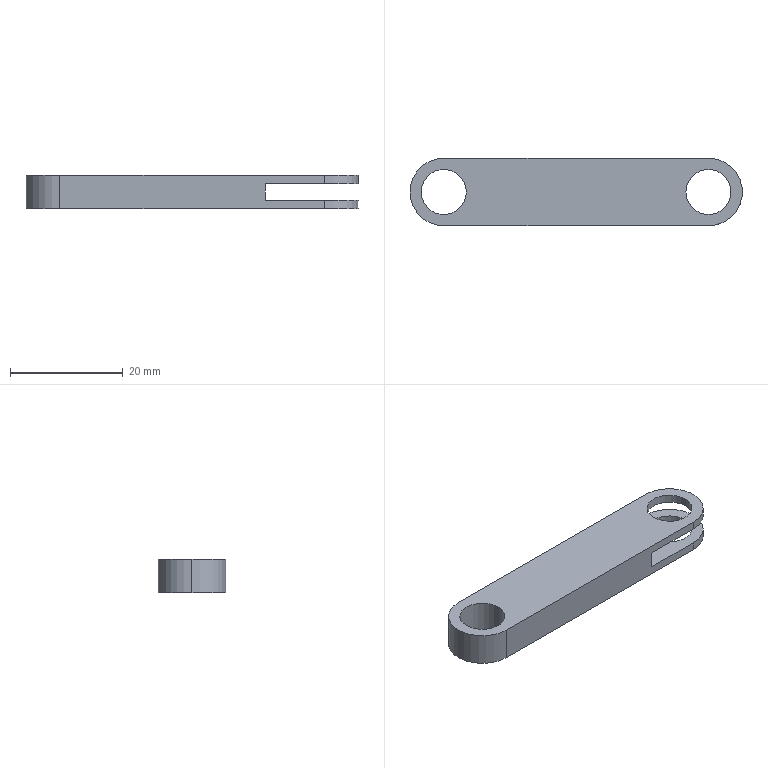Part | SolidWorks | features ICE 2, Extrusion 1 | 1 solid | 17 faces | box 59 x 12 x 6 mm | volume 3063 mm3 | cylinder 10 | plane 7 | commonest cylinder face diameters 8 x6 12 x4
STEP:
#1=CARTESIAN_POINT('',(-27.5,0.,0.));
#2=VERTEX_POINT('',#1);
#3=CARTESIAN_POINT('',(-19.5,0.,0.));
#4=VERTEX_POINT('',#3);
#5=CARTESIAN_POINT('',(-23.5,0.,0.));
#6=DIRECTION('',(0.,0.,1.));
#7=DIRECTION('',(1.,0.,0.));
#8=AXIS2_PLACEMENT_3D('',#5,#6,#7);
#9=CIRCLE('',#8,4.);
#10=EDGE_CURVE('',#2,#4,#9,.T.);
#11=ORIENTED_EDGE('',*,*,#10,.F.);
#12=CARTESIAN_POINT('',(-27.5,0.,6.));
#13=VERTEX_POINT('',#12);
#14=CARTESIAN_POINT('',(-27.5,0.,-29.));
#15=DIRECTION('',(0.,0.,1.));
#16=VECTOR('',#15,1000.);
#17=LINE('',#14,#16);
#18=EDGE_CURVE('',#2,#13,#17,.T.);
#19=ORIENTED_EDGE('',*,*,#18,.T.);
#20=CARTESIAN_POINT('',(-19.5,0.,6.));
#21=VERTEX_POINT('',#20);
#22=CARTESIAN_POINT('',(-23.5,0.,6.));
#23=DIRECTION('',(0.,0.,1.));
#24=DIRECTION('',(1.,0.,0.));
#25=AXIS2_PLACEMENT_3D('',#22,#23,#24);
#26=CIRCLE('',#25,4.);
#27=EDGE_CURVE('',#13,#21,#26,.T.);
#28=ORIENTED_EDGE('',*,*,#27,.T.);
#29=CARTESIAN_POINT('',(-19.5,0.,-29.));
#30=DIRECTION('',(0.,0.,1.));
#31=VECTOR('',#30,1000.);
#32=LINE('',#29,#31);
#33=EDGE_CURVE('',#4,#21,#32,.T.);
#34=ORIENTED_EDGE('',*,*,#33,.F.);
#35=EDGE_LOOP('',(#11,#19,#28,#34));
#36=FACE_OUTER_BOUND('',#35,.T.);
#37=CARTESIAN_POINT('',(-23.5,0.,-29.));
#38=DIRECTION('',(0.,0.,1.));
#39=DIRECTION('',(1.,0.,0.));
#40=AXIS2_PLACEMENT_3D('',#37,#38,#39);
#41=CYLINDRICAL_SURFACE('',#40,4.);
#42=ADVANCED_FACE('',(#36),#41,.F.);
#43=CARTESIAN_POINT('',(19.5,0.,4.5));
#44=VERTEX_POINT('',#43);
#45=CARTESIAN_POINT('',(27.5,0.,4.5));
#46=VERTEX_POINT('',#45);
#47=CARTESIAN_POINT('',(23.5,0.,4.5));
#48=DIRECTION('',(0.,0.,1.));
#49=DIRECTION('',(1.,0.,0.));
#50=AXIS2_PLACEMENT_3D('',#47,#48,#49);
#51=CIRCLE('',#50,4.);
#52=EDGE_CURVE('',#44,#46,#51,.T.);
#53=ORIENTED_EDGE('',*,*,#52,.F.);
#54=CARTESIAN_POINT('',(19.5,0.,6.));
#55=VERTEX_POINT('',#54);
#56=CARTESIAN_POINT('',(19.5,0.,-29.));
#57=DIRECTION('',(0.,0.,1.));
#58=VECTOR('',#57,1000.);
#59=LINE('',#56,#58);
#60=EDGE_CURVE('',#44,#55,#59,.T.);
#61=ORIENTED_EDGE('',*,*,#60,.T.);
#62=CARTESIAN_POINT('',(27.5,0.,6.));
#63=VERTEX_POINT('',#62);
#64=CARTESIAN_POINT('',(23.5,0.,6.));
#65=DIRECTION('',(0.,0.,1.));
#66=DIRECTION('',(1.,0.,0.));
#67=AXIS2_PLACEMENT_3D('',#64,#65,#66);
#68=CIRCLE('',#67,4.);
#69=EDGE_CURVE('',#55,#63,#68,.T.);
#70=ORIENTED_EDGE('',*,*,#69,.T.);
#71=CARTESIAN_POINT('',(27.5,0.,-29.));
#72=DIRECTION('',(0.,0.,1.));
#73=VECTOR('',#72,1000.);
#74=LINE('',#71,#73);
#75=EDGE_CURVE('',#46,#63,#74,.T.);
#76=ORIENTED_EDGE('',*,*,#75,.F.);
#77=EDGE_LOOP('',(#53,#61,#70,#76));
#78=FACE_OUTER_BOUND('',#77,.T.);
#79=CARTESIAN_POINT('',(23.5,0.,-29.));
#80=DIRECTION('',(0.,0.,1.));
#81=DIRECTION('',(1.,0.,0.));
#82=AXIS2_PLACEMENT_3D('',#79,#80,#81);
#83=CYLINDRICAL_SURFACE('',#82,4.);
#84=ADVANCED_FACE('',(#78),#83,.F.);
#85=CARTESIAN_POINT('',(19.5,0.,0.));
#86=VERTEX_POINT('',#85);
#87=CARTESIAN_POINT('',(27.5,0.,0.));
#88=VERTEX_POINT('',#87);
#89=CARTESIAN_POINT('',(23.5,0.,0.));
#90=DIRECTION('',(0.,0.,1.));
#91=DIRECTION('',(1.,0.,0.));
#92=AXIS2_PLACEMENT_3D('',#89,#90,#91);
#93=CIRCLE('',#92,4.);
#94=EDGE_CURVE('',#86,#88,#93,.T.);
#95=ORIENTED_EDGE('',*,*,#94,.F.);
#96=CARTESIAN_POINT('',(19.5,0.,1.5));
#97=VERTEX_POINT('',#96);
#98=CARTESIAN_POINT('',(19.5,0.,-29.));
#99=DIRECTION('',(0.,0.,1.));
#100=VECTOR('',#99,1000.);
#101=LINE('',#98,#100);
#102=EDGE_CURVE('',#86,#97,#101,.T.);
#103=ORIENTED_EDGE('',*,*,#102,.T.);
#104=CARTESIAN_POINT('',(27.5,0.,1.5));
#105=VERTEX_POINT('',#104);
#106=CARTESIAN_POINT('',(23.5,0.,1.5));
#107=DIRECTION('',(0.,0.,-1.));
#108=DIRECTION('',(-1.,0.,0.));
#109=AXIS2_PLACEMENT_3D('',#106,#107,#108);
#110=CIRCLE('',#109,4.);
#111=EDGE_CURVE('',#105,#97,#110,.T.);
#112=ORIENTED_EDGE('',*,*,#111,.F.);
#113=CARTESIAN_POINT('',(27.5,0.,-29.));
#114=DIRECTION('',(0.,0.,1.));
#115=VECTOR('',#114,1000.);
#116=LINE('',#113,#115);
#117=EDGE_CURVE('',#88,#105,#116,.T.);
#118=ORIENTED_EDGE('',*,*,#117,.F.);
#119=EDGE_LOOP('',(#95,#103,#112,#118));
#120=FACE_OUTER_BOUND('',#119,.T.);
#121=CARTESIAN_POINT('',(23.5,0.,-29.));
#122=DIRECTION('',(0.,0.,1.));
#123=DIRECTION('',(1.,0.,0.));
#124=AXIS2_PLACEMENT_3D('',#121,#122,#123);
#125=CYLINDRICAL_SURFACE('',#124,4.);
#126=ADVANCED_FACE('',(#120),#125,.F.);
#127=CARTESIAN_POINT('',(-29.5,0.,6.));
#128=VERTEX_POINT('',#127);
#129=CARTESIAN_POINT('',(-23.5,-6.,6.));
#130=VERTEX_POINT('',#129);
#131=CARTESIAN_POINT('',(-23.5,0.,6.));
#132=DIRECTION('',(0.,0.,1.));
#133=DIRECTION('',(1.,0.,0.));
#134=AXIS2_PLACEMENT_3D('',#131,#132,#133);
#135=CIRCLE('',#134,6.);
#136=EDGE_CURVE('',#128,#130,#135,.T.);
#137=ORIENTED_EDGE('',*,*,#136,.F.);
#138=CARTESIAN_POINT('',(-29.5,0.,0.));
#139=VERTEX_POINT('',#138);
#140=CARTESIAN_POINT('',(-29.5,0.,6.));
#141=DIRECTION('',(0.,0.,-1.));
#142=VECTOR('',#141,1000.);
#143=LINE('',#140,#142);
#144=EDGE_CURVE('',#128,#139,#143,.T.);
#145=ORIENTED_EDGE('',*,*,#144,.T.);
#146=CARTESIAN_POINT('',(-23.5,-6.,0.));
#147=VERTEX_POINT('',#146);
#148=CARTESIAN_POINT('',(-23.5,0.,0.));
#149=DIRECTION('',(0.,0.,1.));
#150=DIRECTION('',(1.,0.,0.));
#151=AXIS2_PLACEMENT_3D('',#148,#149,#150);
#152=CIRCLE('',#151,6.);
#153=EDGE_CURVE('',#139,#147,#152,.T.);
#154=ORIENTED_EDGE('',*,*,#153,.T.);
#155=CARTESIAN_POINT('',(-23.5,-6.,6.));
#156=DIRECTION('',(0.,0.,-1.));
#157=VECTOR('',#156,1000.);
#158=LINE('',#155,#157);
#159=EDGE_CURVE('',#130,#147,#158,.T.);
#160=ORIENTED_EDGE('',*,*,#159,.F.);
#161=EDGE_LOOP('',(#137,#145,#154,#160));
#162=FACE_OUTER_BOUND('',#161,.T.);
#163=CARTESIAN_POINT('',(-23.5,0.,6.));
#164=DIRECTION('',(0.,0.,-1.));
#165=DIRECTION('',(-1.,0.,0.));
#166=AXIS2_PLACEMENT_3D('',#163,#164,#165);
#167=CYLINDRICAL_SURFACE('',#166,6.);
#168=ADVANCED_FACE('',(#162),#167,.T.);
#169=CARTESIAN_POINT('',(23.5,-6.,6.));
#170=VERTEX_POINT('',#169);
#171=CARTESIAN_POINT('',(23.5,-6.,4.5));
#172=VERTEX_POINT('',#171);
#173=CARTESIAN_POINT('',(23.5,-6.,6.));
#174=DIRECTION('',(0.,0.,-1.));
#175=VECTOR('',#174,1000.);
#176=LINE('',#173,#175);
#177=EDGE_CURVE('',#170,#172,#176,.T.);
#178=ORIENTED_EDGE('',*,*,#177,.T.);
#179=CARTESIAN_POINT('',(23.5,6.,4.5));
#180=VERTEX_POINT('',#179);
#181=CARTESIAN_POINT('',(23.5,0.,4.5));
#182=DIRECTION('',(0.,0.,1.));
#183=DIRECTION('',(1.,0.,0.));
#184=AXIS2_PLACEMENT_3D('',#181,#182,#183);
#185=CIRCLE('',#184,6.);
#186=EDGE_CURVE('',#172,#180,#185,.T.);
#187=ORIENTED_EDGE('',*,*,#186,.T.);
#188=CARTESIAN_POINT('',(23.5,6.,6.));
#189=VERTEX_POINT('',#188);
#190=CARTESIAN_POINT('',(23.5,6.,6.));
#191=DIRECTION('',(0.,0.,-1.));
#192=VECTOR('',#191,1000.);
#193=LINE('',#190,#192);
#194=EDGE_CURVE('',#189,#180,#193,.T.);
#195=ORIENTED_EDGE('',*,*,#194,.F.);
#196=CARTESIAN_POINT('',(23.5,0.,6.));
#197=DIRECTION('',(0.,0.,1.));
#198=DIRECTION('',(1.,0.,0.));
#199=AXIS2_PLACEMENT_3D('',#196,#197,#198);
#200=CIRCLE('',#199,6.);
#201=EDGE_CURVE('',#170,#189,#200,.T.);
#202=ORIENTED_EDGE('',*,*,#201,.F.);
#203=EDGE_LOOP('',(#178,#187,#195,#202));
#204=FACE_OUTER_BOUND('',#203,.T.);
#205=CARTESIAN_POINT('',(23.5,0.,6.));
#206=DIRECTION('',(0.,0.,-1.));
#207=DIRECTION('',(-1.,0.,0.));
#208=AXIS2_PLACEMENT_3D('',#205,#206,#207);
#209=CYLINDRICAL_SURFACE('',#208,6.);
#210=ADVANCED_FACE('',(#204),#209,.T.);
#211=CARTESIAN_POINT('',(23.5,6.,1.5));
#212=VERTEX_POINT('',#211);
#213=CARTESIAN_POINT('',(23.5,6.,0.));
#214=VERTEX_POINT('',#213);
#215=CARTESIAN_POINT('',(23.5,6.,6.));
#216=DIRECTION('',(0.,0.,-1.));
#217=VECTOR('',#216,1000.);
#218=LINE('',#215,#217);
#219=EDGE_CURVE('',#212,#214,#218,.T.);
#220=ORIENTED_EDGE('',*,*,#219,.F.);
#221=CARTESIAN_POINT('',(23.5,-6.,1.5));
#222=VERTEX_POINT('',#221);
#223=CARTESIAN_POINT('',(23.5,0.,1.5));
#224=DIRECTION('',(0.,0.,-1.));
#225=DIRECTION('',(-1.,0.,0.));
#226=AXIS2_PLACEMENT_3D('',#223,#224,#225);
#227=CIRCLE('',#226,6.);
#228=EDGE_CURVE('',#212,#222,#227,.T.);
#229=ORIENTED_EDGE('',*,*,#228,.T.);
#230=CARTESIAN_POINT('',(23.5,-6.,0.));
#231=VERTEX_POINT('',#230);
#232=CARTESIAN_POINT('',(23.5,-6.,6.));
#233=DIRECTION('',(0.,0.,-1.));
#234=VECTOR('',#233,1000.);
#235=LINE('',#232,#234);
#236=EDGE_CURVE('',#222,#231,#235,.T.);
#237=ORIENTED_EDGE('',*,*,#236,.T.);
#238=CARTESIAN_POINT('',(23.5,0.,0.));
#239=DIRECTION('',(0.,0.,1.));
#240=DIRECTION('',(1.,0.,0.));
#241=AXIS2_PLACEMENT_3D('',#238,#239,#240);
#242=CIRCLE('',#241,6.);
#243=EDGE_CURVE('',#231,#214,#242,.T.);
#244=ORIENTED_EDGE('',*,*,#243,.T.);
#245=EDGE_LOOP('',(#220,#229,#237,#244));
#246=FACE_OUTER_BOUND('',#245,.T.);
#247=CARTESIAN_POINT('',(23.5,0.,6.));
#248=DIRECTION('',(0.,0.,-1.));
#249=DIRECTION('',(-1.,0.,0.));
#250=AXIS2_PLACEMENT_3D('',#247,#248,#249);
#251=CYLINDRICAL_SURFACE('',#250,6.);
#252=ADVANCED_FACE('',(#246),#251,.T.);
#253=ORIENTED_EDGE('',*,*,#194,.T.);
#254=CARTESIAN_POINT('',(13.,6.,4.5));
#255=VERTEX_POINT('',#254);
#256=CARTESIAN_POINT('',(13.,6.,4.5));
#257=DIRECTION('',(1.,0.,0.));
#258=VECTOR('',#257,1000.);
#259=LINE('',#256,#258);
#260=EDGE_CURVE('',#255,#180,#259,.T.);
#261=ORIENTED_EDGE('',*,*,#260,.F.);
#262=CARTESIAN_POINT('',(13.,6.,1.5));
#263=VERTEX_POINT('',#262);
#264=CARTESIAN_POINT('',(13.,6.,1.5));
#265=DIRECTION('',(0.,0.,1.));
#266=VECTOR('',#265,1000.);
#267=LINE('',#264,#266);
#268=EDGE_CURVE('',#263,#255,#267,.T.);
#269=ORIENTED_EDGE('',*,*,#268,.F.);
#270=CARTESIAN_POINT('',(13.,6.,1.5));
#271=DIRECTION('',(-1.,0.,0.));
#272=VECTOR('',#271,1000.);
#273=LINE('',#270,#272);
#274=EDGE_CURVE('',#212,#263,#273,.T.);
#275=ORIENTED_EDGE('',*,*,#274,.F.);
#276=ORIENTED_EDGE('',*,*,#219,.T.);
#277=CARTESIAN_POINT('',(-23.5,6.,0.));
#278=VERTEX_POINT('',#277);
#279=CARTESIAN_POINT('',(23.5,6.,0.));
#280=DIRECTION('',(-1.,0.,0.));
#281=VECTOR('',#280,1000.);
#282=LINE('',#279,#281);
#283=EDGE_CURVE('',#214,#278,#282,.T.);
#284=ORIENTED_EDGE('',*,*,#283,.T.);
#285=CARTESIAN_POINT('',(-23.5,6.,6.));
#286=VERTEX_POINT('',#285);
#287=CARTESIAN_POINT('',(-23.5,6.,6.));
#288=DIRECTION('',(0.,0.,-1.));
#289=VECTOR('',#288,1000.);
#290=LINE('',#287,#289);
#291=EDGE_CURVE('',#286,#278,#290,.T.);
#292=ORIENTED_EDGE('',*,*,#291,.F.);
#293=CARTESIAN_POINT('',(23.5,6.,6.));
#294=DIRECTION('',(-1.,0.,0.));
#295=VECTOR('',#294,1000.);
#296=LINE('',#293,#295);
#297=EDGE_CURVE('',#189,#286,#296,.T.);
#298=ORIENTED_EDGE('',*,*,#297,.F.);
#299=EDGE_LOOP('',(#253,#261,#269,#275,#276,#284,#292,#298));
#300=FACE_OUTER_BOUND('',#299,.T.);
#301=CARTESIAN_POINT('',(23.5,6.,6.));
#302=DIRECTION('',(0.,-1.,0.));
#303=DIRECTION('',(1.,0.,0.));
#304=AXIS2_PLACEMENT_3D('',#301,#302,#303);
#305=PLANE('',#304);
#306=ADVANCED_FACE('',(#300),#305,.F.);
#307=ORIENTED_EDGE('',*,*,#144,.F.);
#308=CARTESIAN_POINT('',(-23.5,0.,6.));
#309=DIRECTION('',(0.,0.,1.));
#310=DIRECTION('',(1.,0.,0.));
#311=AXIS2_PLACEMENT_3D('',#308,#309,#310);
#312=CIRCLE('',#311,6.);
#313=EDGE_CURVE('',#286,#128,#312,.T.);
#314=ORIENTED_EDGE('',*,*,#313,.F.);
#315=ORIENTED_EDGE('',*,*,#291,.T.);
#316=CARTESIAN_POINT('',(-23.5,0.,0.));
#317=DIRECTION('',(0.,0.,1.));
#318=DIRECTION('',(1.,0.,0.));
#319=AXIS2_PLACEMENT_3D('',#316,#317,#318);
#320=CIRCLE('',#319,6.);
#321=EDGE_CURVE('',#278,#139,#320,.T.);
#322=ORIENTED_EDGE('',*,*,#321,.T.);
#323=EDGE_LOOP('',(#307,#314,#315,#322));
#324=FACE_OUTER_BOUND('',#323,.T.);
#325=CARTESIAN_POINT('',(-23.5,0.,6.));
#326=DIRECTION('',(0.,0.,-1.));
#327=DIRECTION('',(-1.,0.,0.));
#328=AXIS2_PLACEMENT_3D('',#325,#326,#327);
#329=CYLINDRICAL_SURFACE('',#328,6.);
#330=ADVANCED_FACE('',(#324),#329,.T.);
#331=CARTESIAN_POINT('',(13.,-6.,1.5));
#332=VERTEX_POINT('',#331);
#333=CARTESIAN_POINT('',(13.,-6.,4.5));
#334=VERTEX_POINT('',#333);
#335=CARTESIAN_POINT('',(13.,-6.,6.));
#336=DIRECTION('',(0.,0.,1.));
#337=VECTOR('',#336,1000.);
#338=LINE('',#335,#337);
#339=EDGE_CURVE('',#332,#334,#338,.T.);
#340=ORIENTED_EDGE('',*,*,#339,.T.);
#341=CARTESIAN_POINT('',(23.5,-6.,4.5));
#342=DIRECTION('',(1.,0.,0.));
#343=VECTOR('',#342,1000.);
#344=LINE('',#341,#343);
#345=EDGE_CURVE('',#334,#172,#344,.T.);
#346=ORIENTED_EDGE('',*,*,#345,.T.);
#347=ORIENTED_EDGE('',*,*,#177,.F.);
#348=CARTESIAN_POINT('',(23.5,-6.,6.));
#349=DIRECTION('',(1.,0.,0.));
#350=VECTOR('',#349,1000.);
#351=LINE('',#348,#350);
#352=EDGE_CURVE('',#130,#170,#351,.T.);
#353=ORIENTED_EDGE('',*,*,#352,.F.);
#354=ORIENTED_EDGE('',*,*,#159,.T.);
#355=CARTESIAN_POINT('',(23.5,-6.,0.));
#356=DIRECTION('',(1.,0.,0.));
#357=VECTOR('',#356,1000.);
#358=LINE('',#355,#357);
#359=EDGE_CURVE('',#147,#231,#358,.T.);
#360=ORIENTED_EDGE('',*,*,#359,.T.);
#361=ORIENTED_EDGE('',*,*,#236,.F.);
#362=CARTESIAN_POINT('',(23.5,-6.,1.5));
#363=DIRECTION('',(-1.,0.,0.));
#364=VECTOR('',#363,1000.);
#365=LINE('',#362,#364);
#366=EDGE_CURVE('',#222,#332,#365,.T.);
#367=ORIENTED_EDGE('',*,*,#366,.T.);
#368=EDGE_LOOP('',(#340,#346,#347,#353,#354,#360,#361,#367));
#369=FACE_OUTER_BOUND('',#368,.T.);
#370=CARTESIAN_POINT('',(23.5,-6.,6.));
#371=DIRECTION('',(0.,1.,0.));
#372=DIRECTION('',(-1.,0.,0.));
#373=AXIS2_PLACEMENT_3D('',#370,#371,#372);
#374=PLANE('',#373);
#375=ADVANCED_FACE('',(#369),#374,.F.);
#376=CARTESIAN_POINT('',(23.5,0.,6.));
#377=DIRECTION('',(0.,0.,1.));
#378=DIRECTION('',(1.,0.,0.));
#379=AXIS2_PLACEMENT_3D('',#376,#377,#378);
#380=CIRCLE('',#379,4.);
#381=EDGE_CURVE('',#63,#55,#380,.T.);
#382=ORIENTED_EDGE('',*,*,#381,.F.);
#383=ORIENTED_EDGE('',*,*,#69,.F.);
#384=EDGE_LOOP('',(#382,#383));
#385=FACE_BOUND('',#384,.T.);
#386=CARTESIAN_POINT('',(-23.5,0.,6.));
#387=DIRECTION('',(0.,0.,1.));
#388=DIRECTION('',(1.,0.,0.));
#389=AXIS2_PLACEMENT_3D('',#386,#387,#388);
#390=CIRCLE('',#389,4.);
#391=EDGE_CURVE('',#21,#13,#390,.T.);
#392=ORIENTED_EDGE('',*,*,#391,.F.);
#393=ORIENTED_EDGE('',*,*,#27,.F.);
#394=EDGE_LOOP('',(#392,#393));
#395=FACE_BOUND('',#394,.T.);
#396=ORIENTED_EDGE('',*,*,#201,.T.);
#397=ORIENTED_EDGE('',*,*,#297,.T.);
#398=ORIENTED_EDGE('',*,*,#313,.T.);
#399=ORIENTED_EDGE('',*,*,#136,.T.);
#400=ORIENTED_EDGE('',*,*,#352,.T.);
#401=EDGE_LOOP('',(#396,#397,#398,#399,#400));
#402=FACE_OUTER_BOUND('',#401,.T.);
#403=CARTESIAN_POINT('',(23.5,0.,6.));
#404=DIRECTION('',(0.,0.,1.));
#405=DIRECTION('',(1.,0.,0.));
#406=AXIS2_PLACEMENT_3D('',#403,#404,#405);
#407=PLANE('',#406);
#408=ADVANCED_FACE('',(#385,#395,#402),#407,.T.);
#409=CARTESIAN_POINT('',(23.5,0.,0.));
#410=DIRECTION('',(0.,0.,1.));
#411=DIRECTION('',(1.,0.,0.));
#412=AXIS2_PLACEMENT_3D('',#409,#410,#411);
#413=CIRCLE('',#412,4.);
#414=EDGE_CURVE('',#88,#86,#413,.T.);
#415=ORIENTED_EDGE('',*,*,#414,.T.);
#416=ORIENTED_EDGE('',*,*,#94,.T.);
#417=EDGE_LOOP('',(#415,#416));
#418=FACE_BOUND('',#417,.T.);
#419=CARTESIAN_POINT('',(-23.5,0.,0.));
#420=DIRECTION('',(0.,0.,1.));
#421=DIRECTION('',(1.,0.,0.));
#422=AXIS2_PLACEMENT_3D('',#419,#420,#421);
#423=CIRCLE('',#422,4.);
#424=EDGE_CURVE('',#4,#2,#423,.T.);
#425=ORIENTED_EDGE('',*,*,#424,.T.);
#426=ORIENTED_EDGE('',*,*,#10,.T.);
#427=EDGE_LOOP('',(#425,#426));
#428=FACE_BOUND('',#427,.T.);
#429=ORIENTED_EDGE('',*,*,#243,.F.);
#430=ORIENTED_EDGE('',*,*,#359,.F.);
#431=ORIENTED_EDGE('',*,*,#153,.F.);
#432=ORIENTED_EDGE('',*,*,#321,.F.);
#433=ORIENTED_EDGE('',*,*,#283,.F.);
#434=EDGE_LOOP('',(#429,#430,#431,#432,#433));
#435=FACE_OUTER_BOUND('',#434,.T.);
#436=CARTESIAN_POINT('',(23.5,0.,0.));
#437=DIRECTION('',(0.,0.,1.));
#438=DIRECTION('',(1.,0.,0.));
#439=AXIS2_PLACEMENT_3D('',#436,#437,#438);
#440=PLANE('',#439);
#441=ADVANCED_FACE('',(#418,#428,#435),#440,.F.);
#442=CARTESIAN_POINT('',(23.5,0.,4.5));
#443=DIRECTION('',(0.,0.,1.));
#444=DIRECTION('',(1.,0.,0.));
#445=AXIS2_PLACEMENT_3D('',#442,#443,#444);
#446=CIRCLE('',#445,4.);
#447=EDGE_CURVE('',#46,#44,#446,.T.);
#448=ORIENTED_EDGE('',*,*,#447,.T.);
#449=ORIENTED_EDGE('',*,*,#52,.T.);
#450=EDGE_LOOP('',(#448,#449));
#451=FACE_BOUND('',#450,.T.);
#452=ORIENTED_EDGE('',*,*,#345,.F.);
#453=CARTESIAN_POINT('',(13.,-29.,4.5));
#454=DIRECTION('',(0.,1.,0.));
#455=VECTOR('',#454,1000.);
#456=LINE('',#453,#455);
#457=EDGE_CURVE('',#334,#255,#456,.T.);
#458=ORIENTED_EDGE('',*,*,#457,.T.);
#459=ORIENTED_EDGE('',*,*,#260,.T.);
#460=ORIENTED_EDGE('',*,*,#186,.F.);
#461=EDGE_LOOP('',(#452,#458,#459,#460));
#462=FACE_OUTER_BOUND('',#461,.T.);
#463=CARTESIAN_POINT('',(13.,-29.,4.5));
#464=DIRECTION('',(0.,0.,1.));
#465=DIRECTION('',(1.,0.,0.));
#466=AXIS2_PLACEMENT_3D('',#463,#464,#465);
#467=PLANE('',#466);
#468=ADVANCED_FACE('',(#451,#462),#467,.F.);
#469=CARTESIAN_POINT('',(13.,-29.,1.5));
#470=DIRECTION('',(0.,1.,0.));
#471=VECTOR('',#470,1000.);
#472=LINE('',#469,#471);
#473=EDGE_CURVE('',#332,#263,#472,.T.);
#474=ORIENTED_EDGE('',*,*,#473,.T.);
#475=ORIENTED_EDGE('',*,*,#268,.T.);
#476=ORIENTED_EDGE('',*,*,#457,.F.);
#477=ORIENTED_EDGE('',*,*,#339,.F.);
#478=EDGE_LOOP('',(#474,#475,#476,#477));
#479=FACE_OUTER_BOUND('',#478,.T.);
#480=CARTESIAN_POINT('',(13.,-29.,1.5));
#481=DIRECTION('',(-1.,0.,0.));
#482=DIRECTION('',(0.,0.,1.));
#483=AXIS2_PLACEMENT_3D('',#480,#481,#482);
#484=PLANE('',#483);
#485=ADVANCED_FACE('',(#479),#484,.F.);
#486=ORIENTED_EDGE('',*,*,#111,.T.);
#487=CARTESIAN_POINT('',(23.5,0.,1.5));
#488=DIRECTION('',(0.,0.,-1.));
#489=DIRECTION('',(-1.,0.,0.));
#490=AXIS2_PLACEMENT_3D('',#487,#488,#489);
#491=CIRCLE('',#490,4.);
#492=EDGE_CURVE('',#97,#105,#491,.T.);
#493=ORIENTED_EDGE('',*,*,#492,.T.);
#494=EDGE_LOOP('',(#486,#493));
#495=FACE_BOUND('',#494,.T.);
#496=ORIENTED_EDGE('',*,*,#274,.T.);
#497=ORIENTED_EDGE('',*,*,#473,.F.);
#498=ORIENTED_EDGE('',*,*,#366,.F.);
#499=ORIENTED_EDGE('',*,*,#228,.F.);
#500=EDGE_LOOP('',(#496,#497,#498,#499));
#501=FACE_OUTER_BOUND('',#500,.T.);
#502=CARTESIAN_POINT('',(13.,-29.,1.5));
#503=DIRECTION('',(0.,0.,-1.));
#504=DIRECTION('',(-1.,0.,0.));
#505=AXIS2_PLACEMENT_3D('',#502,#503,#504);
#506=PLANE('',#505);
#507=ADVANCED_FACE('',(#495,#501),#506,.F.);
#508=ORIENTED_EDGE('',*,*,#102,.F.);
#509=ORIENTED_EDGE('',*,*,#414,.F.);
#510=ORIENTED_EDGE('',*,*,#117,.T.);
#511=ORIENTED_EDGE('',*,*,#492,.F.);
#512=EDGE_LOOP('',(#508,#509,#510,#511));
#513=FACE_OUTER_BOUND('',#512,.T.);
#514=CARTESIAN_POINT('',(23.5,0.,-29.));
#515=DIRECTION('',(0.,0.,1.));
#516=DIRECTION('',(1.,0.,0.));
#517=AXIS2_PLACEMENT_3D('',#514,#515,#516);
#518=CYLINDRICAL_SURFACE('',#517,4.);
#519=ADVANCED_FACE('',(#513),#518,.F.);
#520=ORIENTED_EDGE('',*,*,#60,.F.);
#521=ORIENTED_EDGE('',*,*,#447,.F.);
#522=ORIENTED_EDGE('',*,*,#75,.T.);
#523=ORIENTED_EDGE('',*,*,#381,.T.);
#524=EDGE_LOOP('',(#520,#521,#522,#523));
#525=FACE_OUTER_BOUND('',#524,.T.);
#526=CARTESIAN_POINT('',(23.5,0.,-29.));
#527=DIRECTION('',(0.,0.,1.));
#528=DIRECTION('',(1.,0.,0.));
#529=AXIS2_PLACEMENT_3D('',#526,#527,#528);
#530=CYLINDRICAL_SURFACE('',#529,4.);
#531=ADVANCED_FACE('',(#525),#530,.F.);
#532=ORIENTED_EDGE('',*,*,#18,.F.);
#533=ORIENTED_EDGE('',*,*,#424,.F.);
#534=ORIENTED_EDGE('',*,*,#33,.T.);
#535=ORIENTED_EDGE('',*,*,#391,.T.);
#536=EDGE_LOOP('',(#532,#533,#534,#535));
#537=FACE_OUTER_BOUND('',#536,.T.);
#538=CARTESIAN_POINT('',(-23.5,0.,-29.));
#539=DIRECTION('',(0.,0.,1.));
#540=DIRECTION('',(1.,0.,0.));
#541=AXIS2_PLACEMENT_3D('',#538,#539,#540);
#542=CYLINDRICAL_SURFACE('',#541,4.);
#543=ADVANCED_FACE('',(#537),#542,.F.);
#544=CLOSED_SHELL('',(#42,#84,#126,#168,#210,#252,#306,#330,#375,#408,#441,#468,#485,#507,#519,#531,#543));
#545=MANIFOLD_SOLID_BREP('',#544);
#546=CARTESIAN_POINT('',(0.,0.,0.));
#547=DIRECTION('',(0.,0.,1.));
#548=DIRECTION('',(1.,0.,0.));
#549=AXIS2_PLACEMENT_3D('',#546,#547,#548);
#550=(LENGTH_UNIT()NAMED_UNIT(*)SI_UNIT(.MILLI.,.METRE.));
#551=UNCERTAINTY_MEASURE_WITH_UNIT(LENGTH_MEASURE(0.00001),#550,'','');
#552=(NAMED_UNIT(*)PLANE_ANGLE_UNIT()SI_UNIT($,.RADIAN.));
#553=(NAMED_UNIT(*)SI_UNIT($,.STERADIAN.)SOLID_ANGLE_UNIT());
#554=(GEOMETRIC_REPRESENTATION_CONTEXT(3)GLOBAL_UNCERTAINTY_ASSIGNED_CONTEXT((#551))GLOBAL_UNIT_ASSIGNED_CONTEXT((#550,#552,#553))REPRESENTATION_CONTEXT('',''));
#555=ADVANCED_BREP_SHAPE_REPRESENTATION('',(#545,#549),#554);